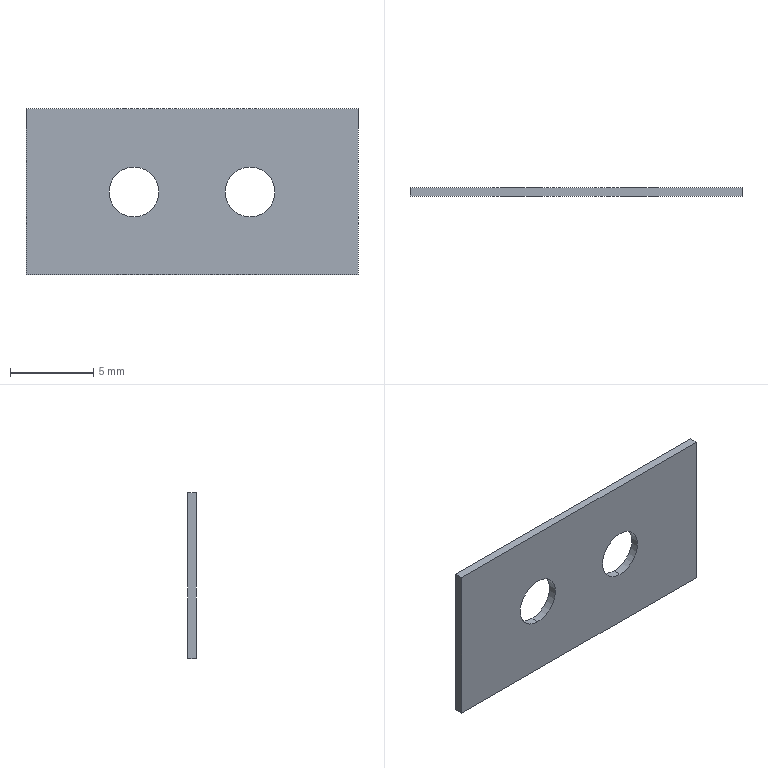Part | SolidWorks | features Extrusion 1 | 1 solid | 10 faces | box 20 x 0.5 x 10 mm | volume 92.931 mm3 | plane 6 | cylinder 4 | commonest cylinder face diameters 3 x4
STEP:
#1=CARTESIAN_POINT('',(3.5,0.5,-1.5));
#2=VERTEX_POINT('',#1);
#3=CARTESIAN_POINT('',(3.5,0.5,1.5));
#4=VERTEX_POINT('',#3);
#5=CARTESIAN_POINT('',(3.5,0.5,0.));
#6=DIRECTION('',(0.,1.,0.));
#7=DIRECTION('',(0.,0.,-1.));
#8=AXIS2_PLACEMENT_3D('',#5,#6,#7);
#9=CIRCLE('',#8,1.5);
#10=EDGE_CURVE('',#2,#4,#9,.T.);
#11=ORIENTED_EDGE('',*,*,#10,.T.);
#12=CARTESIAN_POINT('',(3.5,0.,1.5));
#13=VERTEX_POINT('',#12);
#14=CARTESIAN_POINT('',(3.5,0.5,1.5));
#15=DIRECTION('',(0.,-1.,0.));
#16=VECTOR('',#15,1000.);
#17=LINE('',#14,#16);
#18=EDGE_CURVE('',#4,#13,#17,.T.);
#19=ORIENTED_EDGE('',*,*,#18,.T.);
#20=CARTESIAN_POINT('',(3.5,0.,-1.5));
#21=VERTEX_POINT('',#20);
#22=CARTESIAN_POINT('',(3.5,0.,0.));
#23=DIRECTION('',(0.,1.,0.));
#24=DIRECTION('',(0.,0.,-1.));
#25=AXIS2_PLACEMENT_3D('',#22,#23,#24);
#26=CIRCLE('',#25,1.5);
#27=EDGE_CURVE('',#21,#13,#26,.T.);
#28=ORIENTED_EDGE('',*,*,#27,.F.);
#29=CARTESIAN_POINT('',(3.5,0.5,-1.5));
#30=DIRECTION('',(0.,-1.,0.));
#31=VECTOR('',#30,1000.);
#32=LINE('',#29,#31);
#33=EDGE_CURVE('',#2,#21,#32,.T.);
#34=ORIENTED_EDGE('',*,*,#33,.F.);
#35=EDGE_LOOP('',(#11,#19,#28,#34));
#36=FACE_OUTER_BOUND('',#35,.T.);
#37=CARTESIAN_POINT('',(3.5,0.5,0.));
#38=DIRECTION('',(0.,-1.,0.));
#39=DIRECTION('',(0.,0.,-1.));
#40=AXIS2_PLACEMENT_3D('',#37,#38,#39);
#41=CYLINDRICAL_SURFACE('',#40,1.5);
#42=ADVANCED_FACE('',(#36),#41,.F.);
#43=CARTESIAN_POINT('',(-3.5,0.5,-1.5));
#44=VERTEX_POINT('',#43);
#45=CARTESIAN_POINT('',(-3.5,0.5,1.5));
#46=VERTEX_POINT('',#45);
#47=CARTESIAN_POINT('',(-3.5,0.5,0.));
#48=DIRECTION('',(0.,1.,0.));
#49=DIRECTION('',(0.,0.,1.));
#50=AXIS2_PLACEMENT_3D('',#47,#48,#49);
#51=CIRCLE('',#50,1.5);
#52=EDGE_CURVE('',#44,#46,#51,.T.);
#53=ORIENTED_EDGE('',*,*,#52,.T.);
#54=CARTESIAN_POINT('',(-3.5,0.,1.5));
#55=VERTEX_POINT('',#54);
#56=CARTESIAN_POINT('',(-3.5,0.5,1.5));
#57=DIRECTION('',(0.,-1.,0.));
#58=VECTOR('',#57,1000.);
#59=LINE('',#56,#58);
#60=EDGE_CURVE('',#46,#55,#59,.T.);
#61=ORIENTED_EDGE('',*,*,#60,.T.);
#62=CARTESIAN_POINT('',(-3.5,0.,-1.5));
#63=VERTEX_POINT('',#62);
#64=CARTESIAN_POINT('',(-3.5,0.,0.));
#65=DIRECTION('',(0.,1.,0.));
#66=DIRECTION('',(0.,0.,1.));
#67=AXIS2_PLACEMENT_3D('',#64,#65,#66);
#68=CIRCLE('',#67,1.5);
#69=EDGE_CURVE('',#63,#55,#68,.T.);
#70=ORIENTED_EDGE('',*,*,#69,.F.);
#71=CARTESIAN_POINT('',(-3.5,0.5,-1.5));
#72=DIRECTION('',(0.,-1.,0.));
#73=VECTOR('',#72,1000.);
#74=LINE('',#71,#73);
#75=EDGE_CURVE('',#44,#63,#74,.T.);
#76=ORIENTED_EDGE('',*,*,#75,.F.);
#77=EDGE_LOOP('',(#53,#61,#70,#76));
#78=FACE_OUTER_BOUND('',#77,.T.);
#79=CARTESIAN_POINT('',(-3.5,0.5,0.));
#80=DIRECTION('',(0.,-1.,0.));
#81=DIRECTION('',(0.,0.,-1.));
#82=AXIS2_PLACEMENT_3D('',#79,#80,#81);
#83=CYLINDRICAL_SURFACE('',#82,1.5);
#84=ADVANCED_FACE('',(#78),#83,.F.);
#85=ORIENTED_EDGE('',*,*,#52,.F.);
#86=CARTESIAN_POINT('',(-3.5,0.5,0.));
#87=DIRECTION('',(0.,1.,0.));
#88=DIRECTION('',(0.,0.,1.));
#89=AXIS2_PLACEMENT_3D('',#86,#87,#88);
#90=CIRCLE('',#89,1.5);
#91=EDGE_CURVE('',#46,#44,#90,.T.);
#92=ORIENTED_EDGE('',*,*,#91,.F.);
#93=EDGE_LOOP('',(#85,#92));
#94=FACE_BOUND('',#93,.T.);
#95=CARTESIAN_POINT('',(10.,0.5,5.));
#96=VERTEX_POINT('',#95);
#97=CARTESIAN_POINT('',(10.,0.5,-5.));
#98=VERTEX_POINT('',#97);
#99=CARTESIAN_POINT('',(10.,0.5,5.));
#100=DIRECTION('',(0.,0.,-1.));
#101=VECTOR('',#100,1000.);
#102=LINE('',#99,#101);
#103=EDGE_CURVE('',#96,#98,#102,.T.);
#104=ORIENTED_EDGE('',*,*,#103,.T.);
#105=CARTESIAN_POINT('',(-10.,0.5,-5.));
#106=VERTEX_POINT('',#105);
#107=CARTESIAN_POINT('',(-10.,0.5,-5.));
#108=DIRECTION('',(-1.,0.,0.));
#109=VECTOR('',#108,1000.);
#110=LINE('',#107,#109);
#111=EDGE_CURVE('',#98,#106,#110,.T.);
#112=ORIENTED_EDGE('',*,*,#111,.T.);
#113=CARTESIAN_POINT('',(-10.,0.5,5.));
#114=VERTEX_POINT('',#113);
#115=CARTESIAN_POINT('',(-10.,0.5,5.));
#116=DIRECTION('',(0.,0.,1.));
#117=VECTOR('',#116,1000.);
#118=LINE('',#115,#117);
#119=EDGE_CURVE('',#106,#114,#118,.T.);
#120=ORIENTED_EDGE('',*,*,#119,.T.);
#121=CARTESIAN_POINT('',(-10.,0.5,5.));
#122=DIRECTION('',(1.,0.,0.));
#123=VECTOR('',#122,1000.);
#124=LINE('',#121,#123);
#125=EDGE_CURVE('',#114,#96,#124,.T.);
#126=ORIENTED_EDGE('',*,*,#125,.T.);
#127=EDGE_LOOP('',(#104,#112,#120,#126));
#128=FACE_OUTER_BOUND('',#127,.T.);
#129=ORIENTED_EDGE('',*,*,#10,.F.);
#130=CARTESIAN_POINT('',(3.5,0.5,0.));
#131=DIRECTION('',(0.,1.,0.));
#132=DIRECTION('',(0.,0.,-1.));
#133=AXIS2_PLACEMENT_3D('',#130,#131,#132);
#134=CIRCLE('',#133,1.5);
#135=EDGE_CURVE('',#4,#2,#134,.T.);
#136=ORIENTED_EDGE('',*,*,#135,.F.);
#137=EDGE_LOOP('',(#129,#136));
#138=FACE_BOUND('',#137,.T.);
#139=CARTESIAN_POINT('',(0.,0.5,0.));
#140=DIRECTION('',(0.,-1.,0.));
#141=DIRECTION('',(0.,0.,-1.));
#142=AXIS2_PLACEMENT_3D('',#139,#140,#141);
#143=PLANE('',#142);
#144=ADVANCED_FACE('',(#94,#128,#138),#143,.F.);
#145=ORIENTED_EDGE('',*,*,#69,.T.);
#146=CARTESIAN_POINT('',(-3.5,0.,0.));
#147=DIRECTION('',(0.,1.,0.));
#148=DIRECTION('',(0.,0.,1.));
#149=AXIS2_PLACEMENT_3D('',#146,#147,#148);
#150=CIRCLE('',#149,1.5);
#151=EDGE_CURVE('',#55,#63,#150,.T.);
#152=ORIENTED_EDGE('',*,*,#151,.T.);
#153=EDGE_LOOP('',(#145,#152));
#154=FACE_BOUND('',#153,.T.);
#155=CARTESIAN_POINT('',(10.,0.,5.));
#156=VERTEX_POINT('',#155);
#157=CARTESIAN_POINT('',(10.,0.,-5.));
#158=VERTEX_POINT('',#157);
#159=CARTESIAN_POINT('',(10.,0.,5.));
#160=DIRECTION('',(0.,0.,-1.));
#161=VECTOR('',#160,1000.);
#162=LINE('',#159,#161);
#163=EDGE_CURVE('',#156,#158,#162,.T.);
#164=ORIENTED_EDGE('',*,*,#163,.F.);
#165=CARTESIAN_POINT('',(-10.,0.,5.));
#166=VERTEX_POINT('',#165);
#167=CARTESIAN_POINT('',(-10.,0.,5.));
#168=DIRECTION('',(1.,0.,0.));
#169=VECTOR('',#168,1000.);
#170=LINE('',#167,#169);
#171=EDGE_CURVE('',#166,#156,#170,.T.);
#172=ORIENTED_EDGE('',*,*,#171,.F.);
#173=CARTESIAN_POINT('',(-10.,0.,-5.));
#174=VERTEX_POINT('',#173);
#175=CARTESIAN_POINT('',(-10.,0.,5.));
#176=DIRECTION('',(0.,0.,1.));
#177=VECTOR('',#176,1000.);
#178=LINE('',#175,#177);
#179=EDGE_CURVE('',#174,#166,#178,.T.);
#180=ORIENTED_EDGE('',*,*,#179,.F.);
#181=CARTESIAN_POINT('',(-10.,0.,-5.));
#182=DIRECTION('',(-1.,0.,0.));
#183=VECTOR('',#182,1000.);
#184=LINE('',#181,#183);
#185=EDGE_CURVE('',#158,#174,#184,.T.);
#186=ORIENTED_EDGE('',*,*,#185,.F.);
#187=EDGE_LOOP('',(#164,#172,#180,#186));
#188=FACE_OUTER_BOUND('',#187,.T.);
#189=ORIENTED_EDGE('',*,*,#27,.T.);
#190=CARTESIAN_POINT('',(3.5,0.,0.));
#191=DIRECTION('',(0.,1.,0.));
#192=DIRECTION('',(0.,0.,-1.));
#193=AXIS2_PLACEMENT_3D('',#190,#191,#192);
#194=CIRCLE('',#193,1.5);
#195=EDGE_CURVE('',#13,#21,#194,.T.);
#196=ORIENTED_EDGE('',*,*,#195,.T.);
#197=EDGE_LOOP('',(#189,#196));
#198=FACE_BOUND('',#197,.T.);
#199=CARTESIAN_POINT('',(0.,0.,0.));
#200=DIRECTION('',(0.,-1.,0.));
#201=DIRECTION('',(0.,0.,-1.));
#202=AXIS2_PLACEMENT_3D('',#199,#200,#201);
#203=PLANE('',#202);
#204=ADVANCED_FACE('',(#154,#188,#198),#203,.T.);
#205=ORIENTED_EDGE('',*,*,#163,.T.);
#206=CARTESIAN_POINT('',(10.,0.5,-5.));
#207=DIRECTION('',(0.,-1.,0.));
#208=VECTOR('',#207,1000.);
#209=LINE('',#206,#208);
#210=EDGE_CURVE('',#98,#158,#209,.T.);
#211=ORIENTED_EDGE('',*,*,#210,.F.);
#212=ORIENTED_EDGE('',*,*,#103,.F.);
#213=CARTESIAN_POINT('',(10.,0.5,5.));
#214=DIRECTION('',(0.,-1.,0.));
#215=VECTOR('',#214,1000.);
#216=LINE('',#213,#215);
#217=EDGE_CURVE('',#96,#156,#216,.T.);
#218=ORIENTED_EDGE('',*,*,#217,.T.);
#219=EDGE_LOOP('',(#205,#211,#212,#218));
#220=FACE_OUTER_BOUND('',#219,.T.);
#221=CARTESIAN_POINT('',(10.,0.5,5.));
#222=DIRECTION('',(-1.,0.,0.));
#223=DIRECTION('',(0.,0.,1.));
#224=AXIS2_PLACEMENT_3D('',#221,#222,#223);
#225=PLANE('',#224);
#226=ADVANCED_FACE('',(#220),#225,.F.);
#227=ORIENTED_EDGE('',*,*,#185,.T.);
#228=CARTESIAN_POINT('',(-10.,0.5,-5.));
#229=DIRECTION('',(0.,-1.,0.));
#230=VECTOR('',#229,1000.);
#231=LINE('',#228,#230);
#232=EDGE_CURVE('',#106,#174,#231,.T.);
#233=ORIENTED_EDGE('',*,*,#232,.F.);
#234=ORIENTED_EDGE('',*,*,#111,.F.);
#235=ORIENTED_EDGE('',*,*,#210,.T.);
#236=EDGE_LOOP('',(#227,#233,#234,#235));
#237=FACE_OUTER_BOUND('',#236,.T.);
#238=CARTESIAN_POINT('',(-10.,0.5,-5.));
#239=DIRECTION('',(0.,0.,1.));
#240=DIRECTION('',(1.,0.,0.));
#241=AXIS2_PLACEMENT_3D('',#238,#239,#240);
#242=PLANE('',#241);
#243=ADVANCED_FACE('',(#237),#242,.F.);
#244=ORIENTED_EDGE('',*,*,#179,.T.);
#245=CARTESIAN_POINT('',(-10.,0.5,5.));
#246=DIRECTION('',(0.,-1.,0.));
#247=VECTOR('',#246,1000.);
#248=LINE('',#245,#247);
#249=EDGE_CURVE('',#114,#166,#248,.T.);
#250=ORIENTED_EDGE('',*,*,#249,.F.);
#251=ORIENTED_EDGE('',*,*,#119,.F.);
#252=ORIENTED_EDGE('',*,*,#232,.T.);
#253=EDGE_LOOP('',(#244,#250,#251,#252));
#254=FACE_OUTER_BOUND('',#253,.T.);
#255=CARTESIAN_POINT('',(-10.,0.5,5.));
#256=DIRECTION('',(1.,0.,0.));
#257=DIRECTION('',(0.,0.,-1.));
#258=AXIS2_PLACEMENT_3D('',#255,#256,#257);
#259=PLANE('',#258);
#260=ADVANCED_FACE('',(#254),#259,.F.);
#261=ORIENTED_EDGE('',*,*,#171,.T.);
#262=ORIENTED_EDGE('',*,*,#217,.F.);
#263=ORIENTED_EDGE('',*,*,#125,.F.);
#264=ORIENTED_EDGE('',*,*,#249,.T.);
#265=EDGE_LOOP('',(#261,#262,#263,#264));
#266=FACE_OUTER_BOUND('',#265,.T.);
#267=CARTESIAN_POINT('',(-10.,0.5,5.));
#268=DIRECTION('',(0.,0.,-1.));
#269=DIRECTION('',(-1.,0.,0.));
#270=AXIS2_PLACEMENT_3D('',#267,#268,#269);
#271=PLANE('',#270);
#272=ADVANCED_FACE('',(#266),#271,.F.);
#273=ORIENTED_EDGE('',*,*,#60,.F.);
#274=ORIENTED_EDGE('',*,*,#91,.T.);
#275=ORIENTED_EDGE('',*,*,#75,.T.);
#276=ORIENTED_EDGE('',*,*,#151,.F.);
#277=EDGE_LOOP('',(#273,#274,#275,#276));
#278=FACE_OUTER_BOUND('',#277,.T.);
#279=CARTESIAN_POINT('',(-3.5,0.5,0.));
#280=DIRECTION('',(0.,-1.,0.));
#281=DIRECTION('',(0.,0.,-1.));
#282=AXIS2_PLACEMENT_3D('',#279,#280,#281);
#283=CYLINDRICAL_SURFACE('',#282,1.5);
#284=ADVANCED_FACE('',(#278),#283,.F.);
#285=ORIENTED_EDGE('',*,*,#18,.F.);
#286=ORIENTED_EDGE('',*,*,#135,.T.);
#287=ORIENTED_EDGE('',*,*,#33,.T.);
#288=ORIENTED_EDGE('',*,*,#195,.F.);
#289=EDGE_LOOP('',(#285,#286,#287,#288));
#290=FACE_OUTER_BOUND('',#289,.T.);
#291=CARTESIAN_POINT('',(3.5,0.5,0.));
#292=DIRECTION('',(0.,-1.,0.));
#293=DIRECTION('',(0.,0.,-1.));
#294=AXIS2_PLACEMENT_3D('',#291,#292,#293);
#295=CYLINDRICAL_SURFACE('',#294,1.5);
#296=ADVANCED_FACE('',(#290),#295,.F.);
#297=CLOSED_SHELL('',(#42,#84,#144,#204,#226,#243,#260,#272,#284,#296));
#298=MANIFOLD_SOLID_BREP('',#297);
#299=CARTESIAN_POINT('',(0.,0.,0.));
#300=DIRECTION('',(0.,0.,1.));
#301=DIRECTION('',(1.,0.,0.));
#302=AXIS2_PLACEMENT_3D('',#299,#300,#301);
#303=(LENGTH_UNIT()NAMED_UNIT(*)SI_UNIT(.MILLI.,.METRE.));
#304=UNCERTAINTY_MEASURE_WITH_UNIT(LENGTH_MEASURE(0.00001),#303,'','');
#305=(NAMED_UNIT(*)PLANE_ANGLE_UNIT()SI_UNIT($,.RADIAN.));
#306=(NAMED_UNIT(*)SI_UNIT($,.STERADIAN.)SOLID_ANGLE_UNIT());
#307=(GEOMETRIC_REPRESENTATION_CONTEXT(3)GLOBAL_UNCERTAINTY_ASSIGNED_CONTEXT((#304))GLOBAL_UNIT_ASSIGNED_CONTEXT((#303,#305,#306))REPRESENTATION_CONTEXT('',''));
#308=ADVANCED_BREP_SHAPE_REPRESENTATION('',(#298,#302),#307);